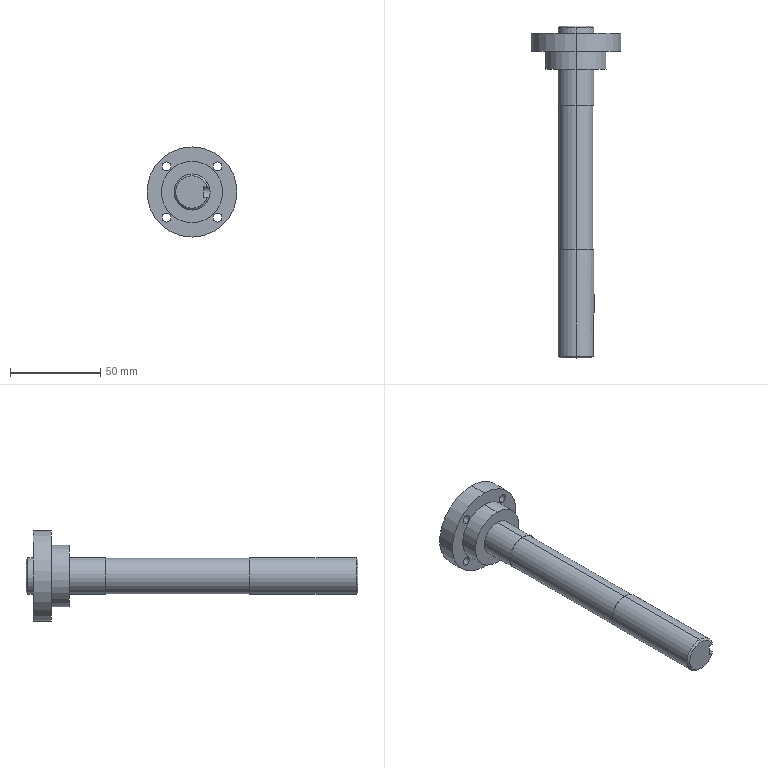Part | STEP file | 0229_213_Shaft | 1 solid | 36 faces | box 50 x 184 x 50 mm | volume 77662 mm3 | cylinder 21 | plane 10 | cone 5 | commonest cylinder face diameters 5 x8 20 x6 19.5 x2 34 x2 50 x2 6 x1